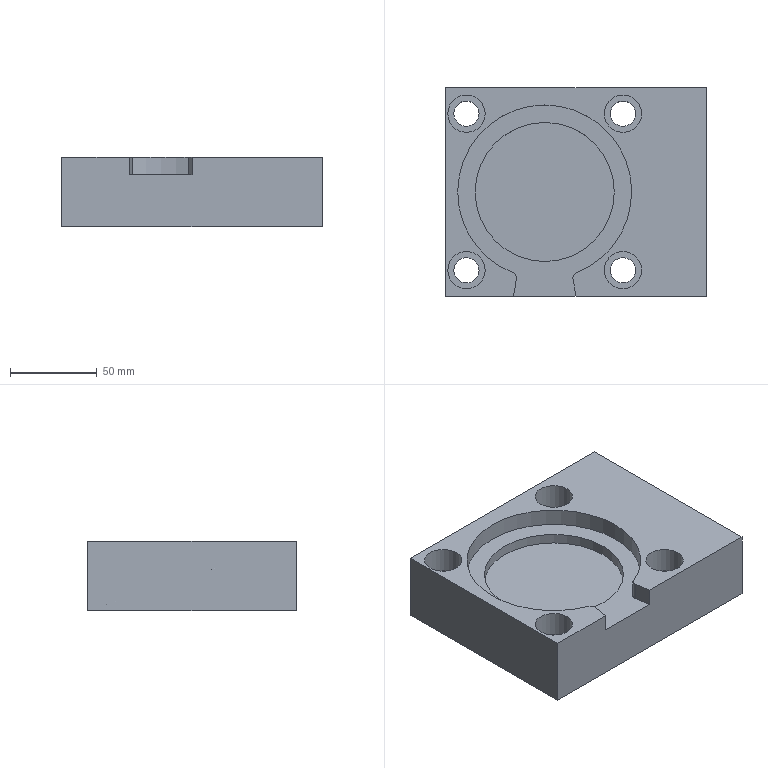CAM job | NX | 3-axis milling, drilling | part box 150 x 120 x 40 mm | stock box 150 x 120 x 40 mm
Tools:
number,name,description,diameter,corner_radius,flute_length,length,flutes
7,D6A45,Milling Tool-5 Parameters,6.0,0.0,3.0,3.0,2
14,14.5ZT,Drilling Tool,14.5,0.0,35.0,50.0,2
10,D10,Milling Tool-5 Parameters,10.0,0.0,50.0,75.0,2
Operations:
program,operation,operation_type,tool,method,geometry_group,spindle_rpm,surface_speed,feed_per_tooth,feed_cut,feed_plunge,cut_length_mm,path_length_mm,cut_time_min,machine_time_min
PROGRAM,DRILLING,Operation,D6A45,METHOD,WORKPIECE,5000.0,94.0,0.025,250.0,0.0,16.0,371.15,0.064,0.0995
PROGRAM,DRILLING_COPY,Operation,14.5ZT,METHOD,WORKPIECE,1200.0,54.0,0.0833,200.0,0.0,189.425,718,0.9471,1.0
PROGRAM,HOLE_MILLING,CylinderMilling,D10,METHOD,WORKPIECE,9500.0,298.0,0.0789,1500.0,100.0,3687.661,4317.661,2.458,2.521
PROGRAM,FLOOR_WALL,VolumeBased25DMillingOperation,D10,METHOD,WORKPIECE,9500.0,298.0,0.1842,3500.0,1000.0,14118.195,14659.003,4.374,4.428
PROGRAM,FLOOR_WALL_COPY,VolumeBased25DMillingOperation,D10,METHOD,WORKPIECE,9500.0,298.0,0.1842,3500.0,1000.0,5044.053,5350.232,1.664,1.694
PROGRAM,FLOOR_WALL_COPY_COPY,VolumeBased25DMillingOperation,D10,METHOD,WORKPIECE,9500.0,298.0,0.0789,1500.0,1000.0,1034.259,1170.586,0.7037,0.7174
PROGRAM,FLOOR_WALL_COPY_COPY_COPY,VolumeBased25DMillingOperation,D10,METHOD,WORKPIECE,9500.0,298.0,0.0789,1500.0,1000.0,773.262,877.637,0.5282,0.5387
PROGRAM,ZLEVEL_PROFILE,ZLevelMilling,D6A45,METHOD,WORKPIECE,9500.0,179.0,0.0737,1400.0,100.0,1540.886,3024.223,1.101,1.249